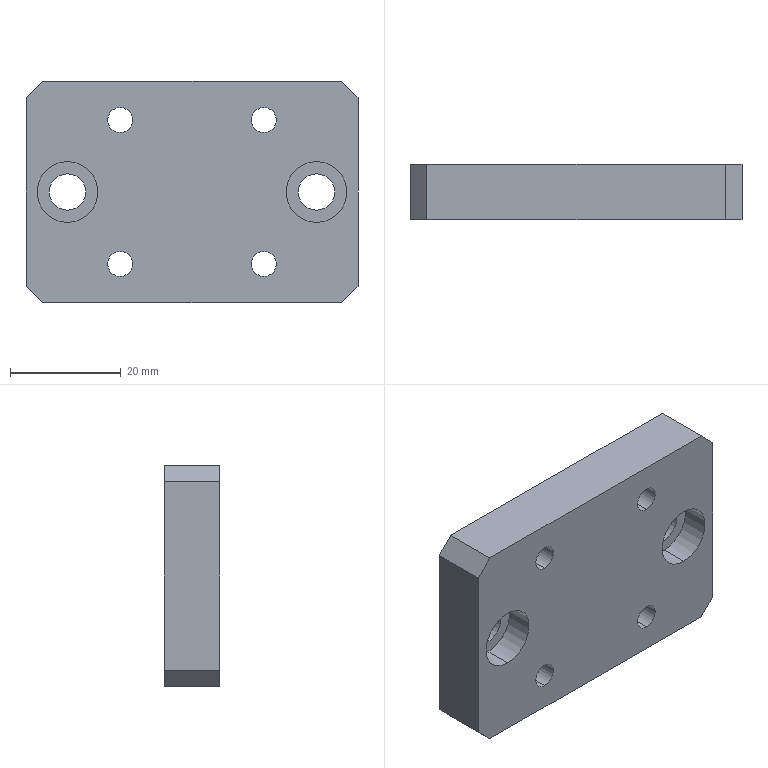Part | SolidWorks | features HoleWzd 2, Chamfer 1, Extrusion 1 | 1 solid | 40 faces | box 60 x 10 x 40 mm | volume 21259 mm3 | cylinder 24 | plane 16 | commonest cylinder face diameters 4.5 x8 8 x8 6.6 x4 11 x4
STEP:
#1=CARTESIAN_POINT('',(22.5,0.,5.5));
#2=VERTEX_POINT('',#1);
#3=CARTESIAN_POINT('',(22.5,0.,-5.5));
#4=VERTEX_POINT('',#3);
#5=CARTESIAN_POINT('',(22.5,0.,0.));
#6=DIRECTION('',(0.,-1.,0.));
#7=DIRECTION('',(0.,0.,-1.));
#8=AXIS2_PLACEMENT_3D('',#5,#6,#7);
#9=CIRCLE('',#8,5.5);
#10=EDGE_CURVE('',#2,#4,#9,.T.);
#11=ORIENTED_EDGE('',*,*,#10,.F.);
#12=CARTESIAN_POINT('',(22.5,-5.,5.5));
#13=VERTEX_POINT('',#12);
#14=CARTESIAN_POINT('',(22.5,-5.,5.5));
#15=DIRECTION('',(0.,-1.,0.));
#16=VECTOR('',#15,1000.);
#17=LINE('',#14,#16);
#18=EDGE_CURVE('',#2,#13,#17,.T.);
#19=ORIENTED_EDGE('',*,*,#18,.T.);
#20=CARTESIAN_POINT('',(22.5,-5.,-5.5));
#21=VERTEX_POINT('',#20);
#22=CARTESIAN_POINT('',(22.5,-5.,0.));
#23=DIRECTION('',(0.,-1.,0.));
#24=DIRECTION('',(0.,0.,-1.));
#25=AXIS2_PLACEMENT_3D('',#22,#23,#24);
#26=CIRCLE('',#25,5.5);
#27=EDGE_CURVE('',#13,#21,#26,.T.);
#28=ORIENTED_EDGE('',*,*,#27,.T.);
#29=CARTESIAN_POINT('',(22.5,-5.,-5.5));
#30=DIRECTION('',(0.,-1.,0.));
#31=VECTOR('',#30,1000.);
#32=LINE('',#29,#31);
#33=EDGE_CURVE('',#4,#21,#32,.T.);
#34=ORIENTED_EDGE('',*,*,#33,.F.);
#35=EDGE_LOOP('',(#11,#19,#28,#34));
#36=FACE_OUTER_BOUND('',#35,.T.);
#37=CARTESIAN_POINT('',(22.5,-5.,0.));
#38=DIRECTION('',(0.,-1.,0.));
#39=DIRECTION('',(0.,0.,-1.));
#40=AXIS2_PLACEMENT_3D('',#37,#38,#39);
#41=CYLINDRICAL_SURFACE('',#40,5.5);
#42=ADVANCED_FACE('',(#36),#41,.F.);
#43=CARTESIAN_POINT('',(22.5,5.,3.3));
#44=VERTEX_POINT('',#43);
#45=CARTESIAN_POINT('',(22.5,5.,-3.3));
#46=VERTEX_POINT('',#45);
#47=CARTESIAN_POINT('',(22.5,5.,0.));
#48=DIRECTION('',(0.,-1.,0.));
#49=DIRECTION('',(0.,0.,-1.));
#50=AXIS2_PLACEMENT_3D('',#47,#48,#49);
#51=CIRCLE('',#50,3.3);
#52=EDGE_CURVE('',#44,#46,#51,.T.);
#53=ORIENTED_EDGE('',*,*,#52,.F.);
#54=CARTESIAN_POINT('',(22.5,0.,3.3));
#55=VERTEX_POINT('',#54);
#56=CARTESIAN_POINT('',(22.5,-5.,3.3));
#57=DIRECTION('',(0.,-1.,0.));
#58=VECTOR('',#57,1000.);
#59=LINE('',#56,#58);
#60=EDGE_CURVE('',#44,#55,#59,.T.);
#61=ORIENTED_EDGE('',*,*,#60,.T.);
#62=CARTESIAN_POINT('',(22.5,0.,-3.3));
#63=VERTEX_POINT('',#62);
#64=CARTESIAN_POINT('',(22.5,0.,0.));
#65=DIRECTION('',(0.,-1.,0.));
#66=DIRECTION('',(0.,0.,-1.));
#67=AXIS2_PLACEMENT_3D('',#64,#65,#66);
#68=CIRCLE('',#67,3.3);
#69=EDGE_CURVE('',#55,#63,#68,.T.);
#70=ORIENTED_EDGE('',*,*,#69,.T.);
#71=CARTESIAN_POINT('',(22.5,-5.,-3.3));
#72=DIRECTION('',(0.,-1.,0.));
#73=VECTOR('',#72,1000.);
#74=LINE('',#71,#73);
#75=EDGE_CURVE('',#46,#63,#74,.T.);
#76=ORIENTED_EDGE('',*,*,#75,.F.);
#77=EDGE_LOOP('',(#53,#61,#70,#76));
#78=FACE_OUTER_BOUND('',#77,.T.);
#79=CARTESIAN_POINT('',(22.5,-5.,0.));
#80=DIRECTION('',(0.,-1.,0.));
#81=DIRECTION('',(0.,0.,-1.));
#82=AXIS2_PLACEMENT_3D('',#79,#80,#81);
#83=CYLINDRICAL_SURFACE('',#82,3.3);
#84=ADVANCED_FACE('',(#78),#83,.F.);
#85=CARTESIAN_POINT('',(-22.5,0.,5.5));
#86=VERTEX_POINT('',#85);
#87=CARTESIAN_POINT('',(-22.5,0.,-5.5));
#88=VERTEX_POINT('',#87);
#89=CARTESIAN_POINT('',(-22.5,0.,0.));
#90=DIRECTION('',(0.,-1.,0.));
#91=DIRECTION('',(0.,0.,-1.));
#92=AXIS2_PLACEMENT_3D('',#89,#90,#91);
#93=CIRCLE('',#92,5.5);
#94=EDGE_CURVE('',#86,#88,#93,.T.);
#95=ORIENTED_EDGE('',*,*,#94,.F.);
#96=CARTESIAN_POINT('',(-22.5,-5.,5.5));
#97=VERTEX_POINT('',#96);
#98=CARTESIAN_POINT('',(-22.5,-5.,5.5));
#99=DIRECTION('',(0.,-1.,0.));
#100=VECTOR('',#99,1000.);
#101=LINE('',#98,#100);
#102=EDGE_CURVE('',#86,#97,#101,.T.);
#103=ORIENTED_EDGE('',*,*,#102,.T.);
#104=CARTESIAN_POINT('',(-22.5,-5.,-5.5));
#105=VERTEX_POINT('',#104);
#106=CARTESIAN_POINT('',(-22.5,-5.,0.));
#107=DIRECTION('',(0.,-1.,0.));
#108=DIRECTION('',(0.,0.,-1.));
#109=AXIS2_PLACEMENT_3D('',#106,#107,#108);
#110=CIRCLE('',#109,5.5);
#111=EDGE_CURVE('',#97,#105,#110,.T.);
#112=ORIENTED_EDGE('',*,*,#111,.T.);
#113=CARTESIAN_POINT('',(-22.5,-5.,-5.5));
#114=DIRECTION('',(0.,-1.,0.));
#115=VECTOR('',#114,1000.);
#116=LINE('',#113,#115);
#117=EDGE_CURVE('',#88,#105,#116,.T.);
#118=ORIENTED_EDGE('',*,*,#117,.F.);
#119=EDGE_LOOP('',(#95,#103,#112,#118));
#120=FACE_OUTER_BOUND('',#119,.T.);
#121=CARTESIAN_POINT('',(-22.5,-5.,0.));
#122=DIRECTION('',(0.,-1.,0.));
#123=DIRECTION('',(0.,0.,-1.));
#124=AXIS2_PLACEMENT_3D('',#121,#122,#123);
#125=CYLINDRICAL_SURFACE('',#124,5.5);
#126=ADVANCED_FACE('',(#120),#125,.F.);
#127=CARTESIAN_POINT('',(-22.5,5.,3.3));
#128=VERTEX_POINT('',#127);
#129=CARTESIAN_POINT('',(-22.5,5.,-3.3));
#130=VERTEX_POINT('',#129);
#131=CARTESIAN_POINT('',(-22.5,5.,0.));
#132=DIRECTION('',(0.,-1.,0.));
#133=DIRECTION('',(0.,0.,-1.));
#134=AXIS2_PLACEMENT_3D('',#131,#132,#133);
#135=CIRCLE('',#134,3.3);
#136=EDGE_CURVE('',#128,#130,#135,.T.);
#137=ORIENTED_EDGE('',*,*,#136,.F.);
#138=CARTESIAN_POINT('',(-22.5,0.,3.3));
#139=VERTEX_POINT('',#138);
#140=CARTESIAN_POINT('',(-22.5,-5.,3.3));
#141=DIRECTION('',(0.,-1.,0.));
#142=VECTOR('',#141,1000.);
#143=LINE('',#140,#142);
#144=EDGE_CURVE('',#128,#139,#143,.T.);
#145=ORIENTED_EDGE('',*,*,#144,.T.);
#146=CARTESIAN_POINT('',(-22.5,0.,-3.3));
#147=VERTEX_POINT('',#146);
#148=CARTESIAN_POINT('',(-22.5,0.,0.));
#149=DIRECTION('',(0.,-1.,0.));
#150=DIRECTION('',(0.,0.,-1.));
#151=AXIS2_PLACEMENT_3D('',#148,#149,#150);
#152=CIRCLE('',#151,3.3);
#153=EDGE_CURVE('',#139,#147,#152,.T.);
#154=ORIENTED_EDGE('',*,*,#153,.T.);
#155=CARTESIAN_POINT('',(-22.5,-5.,-3.3));
#156=DIRECTION('',(0.,-1.,0.));
#157=VECTOR('',#156,1000.);
#158=LINE('',#155,#157);
#159=EDGE_CURVE('',#130,#147,#158,.T.);
#160=ORIENTED_EDGE('',*,*,#159,.F.);
#161=EDGE_LOOP('',(#137,#145,#154,#160));
#162=FACE_OUTER_BOUND('',#161,.T.);
#163=CARTESIAN_POINT('',(-22.5,-5.,0.));
#164=DIRECTION('',(0.,-1.,0.));
#165=DIRECTION('',(0.,0.,-1.));
#166=AXIS2_PLACEMENT_3D('',#163,#164,#165);
#167=CYLINDRICAL_SURFACE('',#166,3.3);
#168=ADVANCED_FACE('',(#162),#167,.F.);
#169=CARTESIAN_POINT('',(13.,0.4,9.));
#170=VERTEX_POINT('',#169);
#171=CARTESIAN_POINT('',(13.,0.4,17.));
#172=VERTEX_POINT('',#171);
#173=CARTESIAN_POINT('',(13.,0.4,13.));
#174=DIRECTION('',(0.,1.,0.));
#175=DIRECTION('',(0.,0.,1.));
#176=AXIS2_PLACEMENT_3D('',#173,#174,#175);
#177=CIRCLE('',#176,4.);
#178=EDGE_CURVE('',#170,#172,#177,.T.);
#179=ORIENTED_EDGE('',*,*,#178,.F.);
#180=CARTESIAN_POINT('',(13.,5.,9.));
#181=VERTEX_POINT('',#180);
#182=CARTESIAN_POINT('',(13.,5.,9.));
#183=DIRECTION('',(0.,1.,0.));
#184=VECTOR('',#183,1000.);
#185=LINE('',#182,#184);
#186=EDGE_CURVE('',#170,#181,#185,.T.);
#187=ORIENTED_EDGE('',*,*,#186,.T.);
#188=CARTESIAN_POINT('',(13.,5.,17.));
#189=VERTEX_POINT('',#188);
#190=CARTESIAN_POINT('',(13.,5.,13.));
#191=DIRECTION('',(0.,1.,0.));
#192=DIRECTION('',(0.,0.,1.));
#193=AXIS2_PLACEMENT_3D('',#190,#191,#192);
#194=CIRCLE('',#193,4.);
#195=EDGE_CURVE('',#181,#189,#194,.T.);
#196=ORIENTED_EDGE('',*,*,#195,.T.);
#197=CARTESIAN_POINT('',(13.,5.,17.));
#198=DIRECTION('',(0.,1.,0.));
#199=VECTOR('',#198,1000.);
#200=LINE('',#197,#199);
#201=EDGE_CURVE('',#172,#189,#200,.T.);
#202=ORIENTED_EDGE('',*,*,#201,.F.);
#203=EDGE_LOOP('',(#179,#187,#196,#202));
#204=FACE_OUTER_BOUND('',#203,.T.);
#205=CARTESIAN_POINT('',(13.,5.,13.));
#206=DIRECTION('',(0.,1.,0.));
#207=DIRECTION('',(0.,0.,1.));
#208=AXIS2_PLACEMENT_3D('',#205,#206,#207);
#209=CYLINDRICAL_SURFACE('',#208,4.);
#210=ADVANCED_FACE('',(#204),#209,.F.);
#211=CARTESIAN_POINT('',(13.,-5.,10.75));
#212=VERTEX_POINT('',#211);
#213=CARTESIAN_POINT('',(13.,-5.,15.25));
#214=VERTEX_POINT('',#213);
#215=CARTESIAN_POINT('',(13.,-5.,13.));
#216=DIRECTION('',(0.,1.,0.));
#217=DIRECTION('',(0.,0.,1.));
#218=AXIS2_PLACEMENT_3D('',#215,#216,#217);
#219=CIRCLE('',#218,2.25);
#220=EDGE_CURVE('',#212,#214,#219,.T.);
#221=ORIENTED_EDGE('',*,*,#220,.F.);
#222=CARTESIAN_POINT('',(13.,0.4,10.75));
#223=VERTEX_POINT('',#222);
#224=CARTESIAN_POINT('',(13.,5.,10.75));
#225=DIRECTION('',(0.,1.,0.));
#226=VECTOR('',#225,1000.);
#227=LINE('',#224,#226);
#228=EDGE_CURVE('',#212,#223,#227,.T.);
#229=ORIENTED_EDGE('',*,*,#228,.T.);
#230=CARTESIAN_POINT('',(13.,0.4,15.25));
#231=VERTEX_POINT('',#230);
#232=CARTESIAN_POINT('',(13.,0.4,13.));
#233=DIRECTION('',(0.,1.,0.));
#234=DIRECTION('',(0.,0.,1.));
#235=AXIS2_PLACEMENT_3D('',#232,#233,#234);
#236=CIRCLE('',#235,2.25);
#237=EDGE_CURVE('',#223,#231,#236,.T.);
#238=ORIENTED_EDGE('',*,*,#237,.T.);
#239=CARTESIAN_POINT('',(13.,5.,15.25));
#240=DIRECTION('',(0.,1.,0.));
#241=VECTOR('',#240,1000.);
#242=LINE('',#239,#241);
#243=EDGE_CURVE('',#214,#231,#242,.T.);
#244=ORIENTED_EDGE('',*,*,#243,.F.);
#245=EDGE_LOOP('',(#221,#229,#238,#244));
#246=FACE_OUTER_BOUND('',#245,.T.);
#247=CARTESIAN_POINT('',(13.,5.,13.));
#248=DIRECTION('',(0.,1.,0.));
#249=DIRECTION('',(0.,0.,1.));
#250=AXIS2_PLACEMENT_3D('',#247,#248,#249);
#251=CYLINDRICAL_SURFACE('',#250,2.25);
#252=ADVANCED_FACE('',(#246),#251,.F.);
#253=CARTESIAN_POINT('',(13.,0.4,-17.));
#254=VERTEX_POINT('',#253);
#255=CARTESIAN_POINT('',(13.,0.4,-9.));
#256=VERTEX_POINT('',#255);
#257=CARTESIAN_POINT('',(13.,0.4,-13.));
#258=DIRECTION('',(0.,1.,0.));
#259=DIRECTION('',(0.,0.,1.));
#260=AXIS2_PLACEMENT_3D('',#257,#258,#259);
#261=CIRCLE('',#260,4.);
#262=EDGE_CURVE('',#254,#256,#261,.T.);
#263=ORIENTED_EDGE('',*,*,#262,.F.);
#264=CARTESIAN_POINT('',(13.,5.,-17.));
#265=VERTEX_POINT('',#264);
#266=CARTESIAN_POINT('',(13.,5.,-17.));
#267=DIRECTION('',(0.,1.,0.));
#268=VECTOR('',#267,1000.);
#269=LINE('',#266,#268);
#270=EDGE_CURVE('',#254,#265,#269,.T.);
#271=ORIENTED_EDGE('',*,*,#270,.T.);
#272=CARTESIAN_POINT('',(13.,5.,-9.));
#273=VERTEX_POINT('',#272);
#274=CARTESIAN_POINT('',(13.,5.,-13.));
#275=DIRECTION('',(0.,1.,0.));
#276=DIRECTION('',(0.,0.,1.));
#277=AXIS2_PLACEMENT_3D('',#274,#275,#276);
#278=CIRCLE('',#277,4.);
#279=EDGE_CURVE('',#265,#273,#278,.T.);
#280=ORIENTED_EDGE('',*,*,#279,.T.);
#281=CARTESIAN_POINT('',(13.,5.,-9.));
#282=DIRECTION('',(0.,1.,0.));
#283=VECTOR('',#282,1000.);
#284=LINE('',#281,#283);
#285=EDGE_CURVE('',#256,#273,#284,.T.);
#286=ORIENTED_EDGE('',*,*,#285,.F.);
#287=EDGE_LOOP('',(#263,#271,#280,#286));
#288=FACE_OUTER_BOUND('',#287,.T.);
#289=CARTESIAN_POINT('',(13.,5.,-13.));
#290=DIRECTION('',(0.,1.,0.));
#291=DIRECTION('',(0.,0.,1.));
#292=AXIS2_PLACEMENT_3D('',#289,#290,#291);
#293=CYLINDRICAL_SURFACE('',#292,4.);
#294=ADVANCED_FACE('',(#288),#293,.F.);
#295=CARTESIAN_POINT('',(13.,-5.,-15.25));
#296=VERTEX_POINT('',#295);
#297=CARTESIAN_POINT('',(13.,-5.,-10.75));
#298=VERTEX_POINT('',#297);
#299=CARTESIAN_POINT('',(13.,-5.,-13.));
#300=DIRECTION('',(0.,1.,0.));
#301=DIRECTION('',(0.,0.,1.));
#302=AXIS2_PLACEMENT_3D('',#299,#300,#301);
#303=CIRCLE('',#302,2.25);
#304=EDGE_CURVE('',#296,#298,#303,.T.);
#305=ORIENTED_EDGE('',*,*,#304,.F.);
#306=CARTESIAN_POINT('',(13.,0.4,-15.25));
#307=VERTEX_POINT('',#306);
#308=CARTESIAN_POINT('',(13.,5.,-15.25));
#309=DIRECTION('',(0.,1.,0.));
#310=VECTOR('',#309,1000.);
#311=LINE('',#308,#310);
#312=EDGE_CURVE('',#296,#307,#311,.T.);
#313=ORIENTED_EDGE('',*,*,#312,.T.);
#314=CARTESIAN_POINT('',(13.,0.4,-10.75));
#315=VERTEX_POINT('',#314);
#316=CARTESIAN_POINT('',(13.,0.4,-13.));
#317=DIRECTION('',(0.,1.,0.));
#318=DIRECTION('',(0.,0.,1.));
#319=AXIS2_PLACEMENT_3D('',#316,#317,#318);
#320=CIRCLE('',#319,2.25);
#321=EDGE_CURVE('',#307,#315,#320,.T.);
#322=ORIENTED_EDGE('',*,*,#321,.T.);
#323=CARTESIAN_POINT('',(13.,5.,-10.75));
#324=DIRECTION('',(0.,1.,0.));
#325=VECTOR('',#324,1000.);
#326=LINE('',#323,#325);
#327=EDGE_CURVE('',#298,#315,#326,.T.);
#328=ORIENTED_EDGE('',*,*,#327,.F.);
#329=EDGE_LOOP('',(#305,#313,#322,#328));
#330=FACE_OUTER_BOUND('',#329,.T.);
#331=CARTESIAN_POINT('',(13.,5.,-13.));
#332=DIRECTION('',(0.,1.,0.));
#333=DIRECTION('',(0.,0.,1.));
#334=AXIS2_PLACEMENT_3D('',#331,#332,#333);
#335=CYLINDRICAL_SURFACE('',#334,2.25);
#336=ADVANCED_FACE('',(#330),#335,.F.);
#337=CARTESIAN_POINT('',(-13.,0.4,-17.));
#338=VERTEX_POINT('',#337);
#339=CARTESIAN_POINT('',(-13.,0.4,-9.));
#340=VERTEX_POINT('',#339);
#341=CARTESIAN_POINT('',(-13.,0.4,-13.));
#342=DIRECTION('',(0.,1.,0.));
#343=DIRECTION('',(0.,0.,1.));
#344=AXIS2_PLACEMENT_3D('',#341,#342,#343);
#345=CIRCLE('',#344,4.);
#346=EDGE_CURVE('',#338,#340,#345,.T.);
#347=ORIENTED_EDGE('',*,*,#346,.F.);
#348=CARTESIAN_POINT('',(-13.,5.,-17.));
#349=VERTEX_POINT('',#348);
#350=CARTESIAN_POINT('',(-13.,5.,-17.));
#351=DIRECTION('',(0.,1.,0.));
#352=VECTOR('',#351,1000.);
#353=LINE('',#350,#352);
#354=EDGE_CURVE('',#338,#349,#353,.T.);
#355=ORIENTED_EDGE('',*,*,#354,.T.);
#356=CARTESIAN_POINT('',(-13.,5.,-9.));
#357=VERTEX_POINT('',#356);
#358=CARTESIAN_POINT('',(-13.,5.,-13.));
#359=DIRECTION('',(0.,1.,0.));
#360=DIRECTION('',(0.,0.,1.));
#361=AXIS2_PLACEMENT_3D('',#358,#359,#360);
#362=CIRCLE('',#361,4.);
#363=EDGE_CURVE('',#349,#357,#362,.T.);
#364=ORIENTED_EDGE('',*,*,#363,.T.);
#365=CARTESIAN_POINT('',(-13.,5.,-9.));
#366=DIRECTION('',(0.,1.,0.));
#367=VECTOR('',#366,1000.);
#368=LINE('',#365,#367);
#369=EDGE_CURVE('',#340,#357,#368,.T.);
#370=ORIENTED_EDGE('',*,*,#369,.F.);
#371=EDGE_LOOP('',(#347,#355,#364,#370));
#372=FACE_OUTER_BOUND('',#371,.T.);
#373=CARTESIAN_POINT('',(-13.,5.,-13.));
#374=DIRECTION('',(0.,1.,0.));
#375=DIRECTION('',(0.,0.,1.));
#376=AXIS2_PLACEMENT_3D('',#373,#374,#375);
#377=CYLINDRICAL_SURFACE('',#376,4.);
#378=ADVANCED_FACE('',(#372),#377,.F.);
#379=CARTESIAN_POINT('',(-13.,-5.,-15.25));
#380=VERTEX_POINT('',#379);
#381=CARTESIAN_POINT('',(-13.,-5.,-10.75));
#382=VERTEX_POINT('',#381);
#383=CARTESIAN_POINT('',(-13.,-5.,-13.));
#384=DIRECTION('',(0.,1.,0.));
#385=DIRECTION('',(0.,0.,1.));
#386=AXIS2_PLACEMENT_3D('',#383,#384,#385);
#387=CIRCLE('',#386,2.25);
#388=EDGE_CURVE('',#380,#382,#387,.T.);
#389=ORIENTED_EDGE('',*,*,#388,.F.);
#390=CARTESIAN_POINT('',(-13.,0.4,-15.25));
#391=VERTEX_POINT('',#390);
#392=CARTESIAN_POINT('',(-13.,5.,-15.25));
#393=DIRECTION('',(0.,1.,0.));
#394=VECTOR('',#393,1000.);
#395=LINE('',#392,#394);
#396=EDGE_CURVE('',#380,#391,#395,.T.);
#397=ORIENTED_EDGE('',*,*,#396,.T.);
#398=CARTESIAN_POINT('',(-13.,0.4,-10.75));
#399=VERTEX_POINT('',#398);
#400=CARTESIAN_POINT('',(-13.,0.4,-13.));
#401=DIRECTION('',(0.,1.,0.));
#402=DIRECTION('',(0.,0.,1.));
#403=AXIS2_PLACEMENT_3D('',#400,#401,#402);
#404=CIRCLE('',#403,2.25);
#405=EDGE_CURVE('',#391,#399,#404,.T.);
#406=ORIENTED_EDGE('',*,*,#405,.T.);
#407=CARTESIAN_POINT('',(-13.,5.,-10.75));
#408=DIRECTION('',(0.,1.,0.));
#409=VECTOR('',#408,1000.);
#410=LINE('',#407,#409);
#411=EDGE_CURVE('',#382,#399,#410,.T.);
#412=ORIENTED_EDGE('',*,*,#411,.F.);
#413=EDGE_LOOP('',(#389,#397,#406,#412));
#414=FACE_OUTER_BOUND('',#413,.T.);
#415=CARTESIAN_POINT('',(-13.,5.,-13.));
#416=DIRECTION('',(0.,1.,0.));
#417=DIRECTION('',(0.,0.,1.));
#418=AXIS2_PLACEMENT_3D('',#415,#416,#417);
#419=CYLINDRICAL_SURFACE('',#418,2.25);
#420=ADVANCED_FACE('',(#414),#419,.F.);
#421=CARTESIAN_POINT('',(-13.,0.4,9.));
#422=VERTEX_POINT('',#421);
#423=CARTESIAN_POINT('',(-13.,0.4,17.));
#424=VERTEX_POINT('',#423);
#425=CARTESIAN_POINT('',(-13.,0.4,13.));
#426=DIRECTION('',(0.,1.,0.));
#427=DIRECTION('',(0.,0.,1.));
#428=AXIS2_PLACEMENT_3D('',#425,#426,#427);
#429=CIRCLE('',#428,4.);
#430=EDGE_CURVE('',#422,#424,#429,.T.);
#431=ORIENTED_EDGE('',*,*,#430,.F.);
#432=CARTESIAN_POINT('',(-13.,5.,9.));
#433=VERTEX_POINT('',#432);
#434=CARTESIAN_POINT('',(-13.,5.,9.));
#435=DIRECTION('',(0.,1.,0.));
#436=VECTOR('',#435,1000.);
#437=LINE('',#434,#436);
#438=EDGE_CURVE('',#422,#433,#437,.T.);
#439=ORIENTED_EDGE('',*,*,#438,.T.);
#440=CARTESIAN_POINT('',(-13.,5.,17.));
#441=VERTEX_POINT('',#440);
#442=CARTESIAN_POINT('',(-13.,5.,13.));
#443=DIRECTION('',(0.,1.,0.));
#444=DIRECTION('',(0.,0.,1.));
#445=AXIS2_PLACEMENT_3D('',#442,#443,#444);
#446=CIRCLE('',#445,4.);
#447=EDGE_CURVE('',#433,#441,#446,.T.);
#448=ORIENTED_EDGE('',*,*,#447,.T.);
#449=CARTESIAN_POINT('',(-13.,5.,17.));
#450=DIRECTION('',(0.,1.,0.));
#451=VECTOR('',#450,1000.);
#452=LINE('',#449,#451);
#453=EDGE_CURVE('',#424,#441,#452,.T.);
#454=ORIENTED_EDGE('',*,*,#453,.F.);
#455=EDGE_LOOP('',(#431,#439,#448,#454));
#456=FACE_OUTER_BOUND('',#455,.T.);
#457=CARTESIAN_POINT('',(-13.,5.,13.));
#458=DIRECTION('',(0.,1.,0.));
#459=DIRECTION('',(0.,0.,1.));
#460=AXIS2_PLACEMENT_3D('',#457,#458,#459);
#461=CYLINDRICAL_SURFACE('',#460,4.);
#462=ADVANCED_FACE('',(#456),#461,.F.);
#463=CARTESIAN_POINT('',(-13.,-5.,10.75));
#464=VERTEX_POINT('',#463);
#465=CARTESIAN_POINT('',(-13.,-5.,15.25));
#466=VERTEX_POINT('',#465);
#467=CARTESIAN_POINT('',(-13.,-5.,13.));
#468=DIRECTION('',(0.,1.,0.));
#469=DIRECTION('',(0.,0.,1.));
#470=AXIS2_PLACEMENT_3D('',#467,#468,#469);
#471=CIRCLE('',#470,2.25);
#472=EDGE_CURVE('',#464,#466,#471,.T.);
#473=ORIENTED_EDGE('',*,*,#472,.F.);
#474=CARTESIAN_POINT('',(-13.,0.4,10.75));
#475=VERTEX_POINT('',#474);
#476=CARTESIAN_POINT('',(-13.,5.,10.75));
#477=DIRECTION('',(0.,1.,0.));
#478=VECTOR('',#477,1000.);
#479=LINE('',#476,#478);
#480=EDGE_CURVE('',#464,#475,#479,.T.);
#481=ORIENTED_EDGE('',*,*,#480,.T.);
#482=CARTESIAN_POINT('',(-13.,0.4,15.25));
#483=VERTEX_POINT('',#482);
#484=CARTESIAN_POINT('',(-13.,0.4,13.));
#485=DIRECTION('',(0.,1.,0.));
#486=DIRECTION('',(0.,0.,1.));
#487=AXIS2_PLACEMENT_3D('',#484,#485,#486);
#488=CIRCLE('',#487,2.25);
#489=EDGE_CURVE('',#475,#483,#488,.T.);
#490=ORIENTED_EDGE('',*,*,#489,.T.);
#491=CARTESIAN_POINT('',(-13.,5.,15.25));
#492=DIRECTION('',(0.,1.,0.));
#493=VECTOR('',#492,1000.);
#494=LINE('',#491,#493);
#495=EDGE_CURVE('',#466,#483,#494,.T.);
#496=ORIENTED_EDGE('',*,*,#495,.F.);
#497=EDGE_LOOP('',(#473,#481,#490,#496));
#498=FACE_OUTER_BOUND('',#497,.T.);
#499=CARTESIAN_POINT('',(-13.,5.,13.));
#500=DIRECTION('',(0.,1.,0.));
#501=DIRECTION('',(0.,0.,1.));
#502=AXIS2_PLACEMENT_3D('',#499,#500,#501);
#503=CYLINDRICAL_SURFACE('',#502,2.25);
#504=ADVANCED_FACE('',(#498),#503,.F.);
#505=CARTESIAN_POINT('',(30.,5.,17.));
#506=VERTEX_POINT('',#505);
#507=CARTESIAN_POINT('',(30.,5.,-17.));
#508=VERTEX_POINT('',#507);
#509=CARTESIAN_POINT('',(30.,5.,20.));
#510=DIRECTION('',(0.,0.,-1.));
#511=VECTOR('',#510,1000.);
#512=LINE('',#509,#511);
#513=EDGE_CURVE('',#506,#508,#512,.T.);
#514=ORIENTED_EDGE('',*,*,#513,.F.);
#515=CARTESIAN_POINT('',(30.,-5.,17.));
#516=VERTEX_POINT('',#515);
#517=CARTESIAN_POINT('',(30.,5.,17.));
#518=DIRECTION('',(0.,-1.,0.));
#519=VECTOR('',#518,1000.);
#520=LINE('',#517,#519);
#521=EDGE_CURVE('',#506,#516,#520,.T.);
#522=ORIENTED_EDGE('',*,*,#521,.T.);
#523=CARTESIAN_POINT('',(30.,-5.,-17.));
#524=VERTEX_POINT('',#523);
#525=CARTESIAN_POINT('',(30.,-5.,20.));
#526=DIRECTION('',(0.,0.,-1.));
#527=VECTOR('',#526,1000.);
#528=LINE('',#525,#527);
#529=EDGE_CURVE('',#516,#524,#528,.T.);
#530=ORIENTED_EDGE('',*,*,#529,.T.);
#531=CARTESIAN_POINT('',(30.,5.,-17.));
#532=DIRECTION('',(0.,1.,0.));
#533=VECTOR('',#532,1000.);
#534=LINE('',#531,#533);
#535=EDGE_CURVE('',#524,#508,#534,.T.);
#536=ORIENTED_EDGE('',*,*,#535,.T.);
#537=EDGE_LOOP('',(#514,#522,#530,#536));
#538=FACE_OUTER_BOUND('',#537,.T.);
#539=CARTESIAN_POINT('',(30.,5.,20.));
#540=DIRECTION('',(-1.,0.,0.));
#541=DIRECTION('',(0.,0.,1.));
#542=AXIS2_PLACEMENT_3D('',#539,#540,#541);
#543=PLANE('',#542);
#544=ADVANCED_FACE('',(#538),#543,.F.);
#545=CARTESIAN_POINT('',(27.,5.,-20.));
#546=VERTEX_POINT('',#545);
#547=CARTESIAN_POINT('',(-27.,5.,-20.));
#548=VERTEX_POINT('',#547);
#549=CARTESIAN_POINT('',(-30.,5.,-20.));
#550=DIRECTION('',(-1.,0.,0.));
#551=VECTOR('',#550,1000.);
#552=LINE('',#549,#551);
#553=EDGE_CURVE('',#546,#548,#552,.T.);
#554=ORIENTED_EDGE('',*,*,#553,.F.);
#555=CARTESIAN_POINT('',(27.,-5.,-20.));
#556=VERTEX_POINT('',#555);
#557=CARTESIAN_POINT('',(27.,5.,-20.));
#558=DIRECTION('',(0.,-1.,0.));
#559=VECTOR('',#558,1000.);
#560=LINE('',#557,#559);
#561=EDGE_CURVE('',#546,#556,#560,.T.);
#562=ORIENTED_EDGE('',*,*,#561,.T.);
#563=CARTESIAN_POINT('',(-27.,-5.,-20.));
#564=VERTEX_POINT('',#563);
#565=CARTESIAN_POINT('',(-30.,-5.,-20.));
#566=DIRECTION('',(-1.,0.,0.));
#567=VECTOR('',#566,1000.);
#568=LINE('',#565,#567);
#569=EDGE_CURVE('',#556,#564,#568,.T.);
#570=ORIENTED_EDGE('',*,*,#569,.T.);
#571=CARTESIAN_POINT('',(-27.,5.,-20.));
#572=DIRECTION('',(0.,1.,0.));
#573=VECTOR('',#572,1000.);
#574=LINE('',#571,#573);
#575=EDGE_CURVE('',#564,#548,#574,.T.);
#576=ORIENTED_EDGE('',*,*,#575,.T.);
#577=EDGE_LOOP('',(#554,#562,#570,#576));
#578=FACE_OUTER_BOUND('',#577,.T.);
#579=CARTESIAN_POINT('',(-30.,5.,-20.));
#580=DIRECTION('',(0.,0.,1.));
#581=DIRECTION('',(1.,0.,0.));
#582=AXIS2_PLACEMENT_3D('',#579,#580,#581);
#583=PLANE('',#582);
#584=ADVANCED_FACE('',(#578),#583,.F.);
#585=CARTESIAN_POINT('',(-30.,5.,-17.));
#586=VERTEX_POINT('',#585);
#587=CARTESIAN_POINT('',(-30.,5.,17.));
#588=VERTEX_POINT('',#587);
#589=CARTESIAN_POINT('',(-30.,5.,20.));
#590=DIRECTION('',(0.,0.,1.));
#591=VECTOR('',#590,1000.);
#592=LINE('',#589,#591);
#593=EDGE_CURVE('',#586,#588,#592,.T.);
#594=ORIENTED_EDGE('',*,*,#593,.F.);
#595=CARTESIAN_POINT('',(-30.,-5.,-17.));
#596=VERTEX_POINT('',#595);
#597=CARTESIAN_POINT('',(-30.,5.,-17.));
#598=DIRECTION('',(0.,-1.,0.));
#599=VECTOR('',#598,1000.);
#600=LINE('',#597,#599);
#601=EDGE_CURVE('',#586,#596,#600,.T.);
#602=ORIENTED_EDGE('',*,*,#601,.T.);
#603=CARTESIAN_POINT('',(-30.,-5.,17.));
#604=VERTEX_POINT('',#603);
#605=CARTESIAN_POINT('',(-30.,-5.,20.));
#606=DIRECTION('',(0.,0.,1.));
#607=VECTOR('',#606,1000.);
#608=LINE('',#605,#607);
#609=EDGE_CURVE('',#596,#604,#608,.T.);
#610=ORIENTED_EDGE('',*,*,#609,.T.);
#611=CARTESIAN_POINT('',(-30.,5.,17.));
#612=DIRECTION('',(0.,1.,0.));
#613=VECTOR('',#612,1000.);
#614=LINE('',#611,#613);
#615=EDGE_CURVE('',#604,#588,#614,.T.);
#616=ORIENTED_EDGE('',*,*,#615,.T.);
#617=EDGE_LOOP('',(#594,#602,#610,#616));
#618=FACE_OUTER_BOUND('',#617,.T.);
#619=CARTESIAN_POINT('',(-30.,5.,20.));
#620=DIRECTION('',(1.,0.,0.));
#621=DIRECTION('',(0.,0.,-1.));
#622=AXIS2_PLACEMENT_3D('',#619,#620,#621);
#623=PLANE('',#622);
#624=ADVANCED_FACE('',(#618),#623,.F.);
#625=CARTESIAN_POINT('',(-27.,-5.,20.));
#626=VERTEX_POINT('',#625);
#627=CARTESIAN_POINT('',(27.,-5.,20.));
#628=VERTEX_POINT('',#627);
#629=CARTESIAN_POINT('',(-30.,-5.,20.));
#630=DIRECTION('',(1.,0.,0.));
#631=VECTOR('',#630,1000.);
#632=LINE('',#629,#631);
#633=EDGE_CURVE('',#626,#628,#632,.T.);
#634=ORIENTED_EDGE('',*,*,#633,.T.);
#635=CARTESIAN_POINT('',(27.,5.,20.));
#636=VERTEX_POINT('',#635);
#637=CARTESIAN_POINT('',(27.,5.,20.));
#638=DIRECTION('',(0.,1.,0.));
#639=VECTOR('',#638,1000.);
#640=LINE('',#637,#639);
#641=EDGE_CURVE('',#628,#636,#640,.T.);
#642=ORIENTED_EDGE('',*,*,#641,.T.);
#643=CARTESIAN_POINT('',(-27.,5.,20.));
#644=VERTEX_POINT('',#643);
#645=CARTESIAN_POINT('',(-30.,5.,20.));
#646=DIRECTION('',(1.,0.,0.));
#647=VECTOR('',#646,1000.);
#648=LINE('',#645,#647);
#649=EDGE_CURVE('',#644,#636,#648,.T.);
#650=ORIENTED_EDGE('',*,*,#649,.F.);
#651=CARTESIAN_POINT('',(-27.,5.,20.));
#652=DIRECTION('',(0.,-1.,0.));
#653=VECTOR('',#652,1000.);
#654=LINE('',#651,#653);
#655=EDGE_CURVE('',#644,#626,#654,.T.);
#656=ORIENTED_EDGE('',*,*,#655,.T.);
#657=EDGE_LOOP('',(#634,#642,#650,#656));
#658=FACE_OUTER_BOUND('',#657,.T.);
#659=CARTESIAN_POINT('',(-30.,5.,20.));
#660=DIRECTION('',(0.,0.,-1.));
#661=DIRECTION('',(-1.,0.,0.));
#662=AXIS2_PLACEMENT_3D('',#659,#660,#661);
#663=PLANE('',#662);
#664=ADVANCED_FACE('',(#658),#663,.F.);
#665=CARTESIAN_POINT('',(22.5,5.,0.));
#666=DIRECTION('',(0.,-1.,0.));
#667=DIRECTION('',(0.,0.,-1.));
#668=AXIS2_PLACEMENT_3D('',#665,#666,#667);
#669=CIRCLE('',#668,3.3);
#670=EDGE_CURVE('',#46,#44,#669,.T.);
#671=ORIENTED_EDGE('',*,*,#670,.T.);
#672=ORIENTED_EDGE('',*,*,#52,.T.);
#673=EDGE_LOOP('',(#671,#672));
#674=FACE_BOUND('',#673,.T.);
#675=CARTESIAN_POINT('',(-22.5,5.,0.));
#676=DIRECTION('',(0.,-1.,0.));
#677=DIRECTION('',(0.,0.,-1.));
#678=AXIS2_PLACEMENT_3D('',#675,#676,#677);
#679=CIRCLE('',#678,3.3);
#680=EDGE_CURVE('',#130,#128,#679,.T.);
#681=ORIENTED_EDGE('',*,*,#680,.T.);
#682=ORIENTED_EDGE('',*,*,#136,.T.);
#683=EDGE_LOOP('',(#681,#682));
#684=FACE_BOUND('',#683,.T.);
#685=CARTESIAN_POINT('',(13.,5.,13.));
#686=DIRECTION('',(0.,1.,0.));
#687=DIRECTION('',(0.,0.,1.));
#688=AXIS2_PLACEMENT_3D('',#685,#686,#687);
#689=CIRCLE('',#688,4.);
#690=EDGE_CURVE('',#189,#181,#689,.T.);
#691=ORIENTED_EDGE('',*,*,#690,.F.);
#692=ORIENTED_EDGE('',*,*,#195,.F.);
#693=EDGE_LOOP('',(#691,#692));
#694=FACE_BOUND('',#693,.T.);
#695=CARTESIAN_POINT('',(13.,5.,-13.));
#696=DIRECTION('',(0.,1.,0.));
#697=DIRECTION('',(0.,0.,1.));
#698=AXIS2_PLACEMENT_3D('',#695,#696,#697);
#699=CIRCLE('',#698,4.);
#700=EDGE_CURVE('',#273,#265,#699,.T.);
#701=ORIENTED_EDGE('',*,*,#700,.F.);
#702=ORIENTED_EDGE('',*,*,#279,.F.);
#703=EDGE_LOOP('',(#701,#702));
#704=FACE_BOUND('',#703,.T.);
#705=CARTESIAN_POINT('',(-13.,5.,-13.));
#706=DIRECTION('',(0.,1.,0.));
#707=DIRECTION('',(0.,0.,1.));
#708=AXIS2_PLACEMENT_3D('',#705,#706,#707);
#709=CIRCLE('',#708,4.);
#710=EDGE_CURVE('',#357,#349,#709,.T.);
#711=ORIENTED_EDGE('',*,*,#710,.F.);
#712=ORIENTED_EDGE('',*,*,#363,.F.);
#713=EDGE_LOOP('',(#711,#712));
#714=FACE_BOUND('',#713,.T.);
#715=CARTESIAN_POINT('',(-13.,5.,13.));
#716=DIRECTION('',(0.,1.,0.));
#717=DIRECTION('',(0.,0.,1.));
#718=AXIS2_PLACEMENT_3D('',#715,#716,#717);
#719=CIRCLE('',#718,4.);
#720=EDGE_CURVE('',#441,#433,#719,.T.);
#721=ORIENTED_EDGE('',*,*,#720,.F.);
#722=ORIENTED_EDGE('',*,*,#447,.F.);
#723=EDGE_LOOP('',(#721,#722));
#724=FACE_BOUND('',#723,.T.);
#725=ORIENTED_EDGE('',*,*,#649,.T.);
#726=CARTESIAN_POINT('',(30.,5.,17.));
#727=DIRECTION('',(0.7071,0.,-0.7071));
#728=VECTOR('',#727,1000.);
#729=LINE('',#726,#728);
#730=EDGE_CURVE('',#636,#506,#729,.T.);
#731=ORIENTED_EDGE('',*,*,#730,.T.);
#732=ORIENTED_EDGE('',*,*,#513,.T.);
#733=CARTESIAN_POINT('',(27.,5.,-20.));
#734=DIRECTION('',(-0.7071,0.,-0.7071));
#735=VECTOR('',#734,1000.);
#736=LINE('',#733,#735);
#737=EDGE_CURVE('',#508,#546,#736,.T.);
#738=ORIENTED_EDGE('',*,*,#737,.T.);
#739=ORIENTED_EDGE('',*,*,#553,.T.);
#740=CARTESIAN_POINT('',(-30.,5.,-17.));
#741=DIRECTION('',(-0.7071,0.,0.7071));
#742=VECTOR('',#741,1000.);
#743=LINE('',#740,#742);
#744=EDGE_CURVE('',#548,#586,#743,.T.);
#745=ORIENTED_EDGE('',*,*,#744,.T.);
#746=ORIENTED_EDGE('',*,*,#593,.T.);
#747=CARTESIAN_POINT('',(-27.,5.,20.));
#748=DIRECTION('',(0.7071,0.,0.7071));
#749=VECTOR('',#748,1000.);
#750=LINE('',#747,#749);
#751=EDGE_CURVE('',#588,#644,#750,.T.);
#752=ORIENTED_EDGE('',*,*,#751,.T.);
#753=EDGE_LOOP('',(#725,#731,#732,#738,#739,#745,#746,#752));
#754=FACE_OUTER_BOUND('',#753,.T.);
#755=CARTESIAN_POINT('',(0.,5.,0.));
#756=DIRECTION('',(0.,-1.,0.));
#757=DIRECTION('',(0.,0.,-1.));
#758=AXIS2_PLACEMENT_3D('',#755,#756,#757);
#759=PLANE('',#758);
#760=ADVANCED_FACE('',(#674,#684,#694,#704,#714,#724,#754),#759,.F.);
#761=CARTESIAN_POINT('',(22.5,-5.,0.));
#762=DIRECTION('',(0.,-1.,0.));
#763=DIRECTION('',(0.,0.,-1.));
#764=AXIS2_PLACEMENT_3D('',#761,#762,#763);
#765=CIRCLE('',#764,5.5);
#766=EDGE_CURVE('',#21,#13,#765,.T.);
#767=ORIENTED_EDGE('',*,*,#766,.F.);
#768=ORIENTED_EDGE('',*,*,#27,.F.);
#769=EDGE_LOOP('',(#767,#768));
#770=FACE_BOUND('',#769,.T.);
#771=CARTESIAN_POINT('',(-22.5,-5.,0.));
#772=DIRECTION('',(0.,-1.,0.));
#773=DIRECTION('',(0.,0.,-1.));
#774=AXIS2_PLACEMENT_3D('',#771,#772,#773);
#775=CIRCLE('',#774,5.5);
#776=EDGE_CURVE('',#105,#97,#775,.T.);
#777=ORIENTED_EDGE('',*,*,#776,.F.);
#778=ORIENTED_EDGE('',*,*,#111,.F.);
#779=EDGE_LOOP('',(#777,#778));
#780=FACE_BOUND('',#779,.T.);
#781=CARTESIAN_POINT('',(13.,-5.,13.));
#782=DIRECTION('',(0.,1.,0.));
#783=DIRECTION('',(0.,0.,1.));
#784=AXIS2_PLACEMENT_3D('',#781,#782,#783);
#785=CIRCLE('',#784,2.25);
#786=EDGE_CURVE('',#214,#212,#785,.T.);
#787=ORIENTED_EDGE('',*,*,#786,.T.);
#788=ORIENTED_EDGE('',*,*,#220,.T.);
#789=EDGE_LOOP('',(#787,#788));
#790=FACE_BOUND('',#789,.T.);
#791=CARTESIAN_POINT('',(13.,-5.,-13.));
#792=DIRECTION('',(0.,1.,0.));
#793=DIRECTION('',(0.,0.,1.));
#794=AXIS2_PLACEMENT_3D('',#791,#792,#793);
#795=CIRCLE('',#794,2.25);
#796=EDGE_CURVE('',#298,#296,#795,.T.);
#797=ORIENTED_EDGE('',*,*,#796,.T.);
#798=ORIENTED_EDGE('',*,*,#304,.T.);
#799=EDGE_LOOP('',(#797,#798));
#800=FACE_BOUND('',#799,.T.);
#801=CARTESIAN_POINT('',(-13.,-5.,-13.));
#802=DIRECTION('',(0.,1.,0.));
#803=DIRECTION('',(0.,0.,1.));
#804=AXIS2_PLACEMENT_3D('',#801,#802,#803);
#805=CIRCLE('',#804,2.25);
#806=EDGE_CURVE('',#382,#380,#805,.T.);
#807=ORIENTED_EDGE('',*,*,#806,.T.);
#808=ORIENTED_EDGE('',*,*,#388,.T.);
#809=EDGE_LOOP('',(#807,#808));
#810=FACE_BOUND('',#809,.T.);
#811=CARTESIAN_POINT('',(-13.,-5.,13.));
#812=DIRECTION('',(0.,1.,0.));
#813=DIRECTION('',(0.,0.,1.));
#814=AXIS2_PLACEMENT_3D('',#811,#812,#813);
#815=CIRCLE('',#814,2.25);
#816=EDGE_CURVE('',#466,#464,#815,.T.);
#817=ORIENTED_EDGE('',*,*,#816,.T.);
#818=ORIENTED_EDGE('',*,*,#472,.T.);
#819=EDGE_LOOP('',(#817,#818));
#820=FACE_BOUND('',#819,.T.);
#821=ORIENTED_EDGE('',*,*,#529,.F.);
#822=CARTESIAN_POINT('',(23.5,-5.,23.5));
#823=DIRECTION('',(-0.7071,0.,0.7071));
#824=VECTOR('',#823,1000.);
#825=LINE('',#822,#824);
#826=EDGE_CURVE('',#516,#628,#825,.T.);
#827=ORIENTED_EDGE('',*,*,#826,.T.);
#828=ORIENTED_EDGE('',*,*,#633,.F.);
#829=CARTESIAN_POINT('',(-23.5,-5.,23.5));
#830=DIRECTION('',(-0.7071,0.,-0.7071));
#831=VECTOR('',#830,1000.);
#832=LINE('',#829,#831);
#833=EDGE_CURVE('',#626,#604,#832,.T.);
#834=ORIENTED_EDGE('',*,*,#833,.T.);
#835=ORIENTED_EDGE('',*,*,#609,.F.);
#836=CARTESIAN_POINT('',(-23.5,-5.,-23.5));
#837=DIRECTION('',(0.7071,0.,-0.7071));
#838=VECTOR('',#837,1000.);
#839=LINE('',#836,#838);
#840=EDGE_CURVE('',#596,#564,#839,.T.);
#841=ORIENTED_EDGE('',*,*,#840,.T.);
#842=ORIENTED_EDGE('',*,*,#569,.F.);
#843=CARTESIAN_POINT('',(23.5,-5.,-23.5));
#844=DIRECTION('',(0.7071,0.,0.7071));
#845=VECTOR('',#844,1000.);
#846=LINE('',#843,#845);
#847=EDGE_CURVE('',#556,#524,#846,.T.);
#848=ORIENTED_EDGE('',*,*,#847,.T.);
#849=EDGE_LOOP('',(#821,#827,#828,#834,#835,#841,#842,#848));
#850=FACE_OUTER_BOUND('',#849,.T.);
#851=CARTESIAN_POINT('',(0.,-5.,0.));
#852=DIRECTION('',(0.,-1.,0.));
#853=DIRECTION('',(0.,0.,-1.));
#854=AXIS2_PLACEMENT_3D('',#851,#852,#853);
#855=PLANE('',#854);
#856=ADVANCED_FACE('',(#770,#780,#790,#800,#810,#820,#850),#855,.T.);
#857=ORIENTED_EDGE('',*,*,#480,.F.);
#858=ORIENTED_EDGE('',*,*,#816,.F.);
#859=ORIENTED_EDGE('',*,*,#495,.T.);
#860=CARTESIAN_POINT('',(-13.,0.4,13.));
#861=DIRECTION('',(0.,1.,0.));
#862=DIRECTION('',(0.,0.,1.));
#863=AXIS2_PLACEMENT_3D('',#860,#861,#862);
#864=CIRCLE('',#863,2.25);
#865=EDGE_CURVE('',#483,#475,#864,.T.);
#866=ORIENTED_EDGE('',*,*,#865,.T.);
#867=EDGE_LOOP('',(#857,#858,#859,#866));
#868=FACE_OUTER_BOUND('',#867,.T.);
#869=CARTESIAN_POINT('',(-13.,5.,13.));
#870=DIRECTION('',(0.,1.,0.));
#871=DIRECTION('',(0.,0.,1.));
#872=AXIS2_PLACEMENT_3D('',#869,#870,#871);
#873=CYLINDRICAL_SURFACE('',#872,2.25);
#874=ADVANCED_FACE('',(#868),#873,.F.);
#875=ORIENTED_EDGE('',*,*,#865,.F.);
#876=ORIENTED_EDGE('',*,*,#489,.F.);
#877=EDGE_LOOP('',(#875,#876));
#878=FACE_BOUND('',#877,.T.);
#879=CARTESIAN_POINT('',(-13.,0.4,13.));
#880=DIRECTION('',(0.,1.,0.));
#881=DIRECTION('',(0.,0.,1.));
#882=AXIS2_PLACEMENT_3D('',#879,#880,#881);
#883=CIRCLE('',#882,4.);
#884=EDGE_CURVE('',#424,#422,#883,.T.);
#885=ORIENTED_EDGE('',*,*,#884,.T.);
#886=ORIENTED_EDGE('',*,*,#430,.T.);
#887=EDGE_LOOP('',(#885,#886));
#888=FACE_OUTER_BOUND('',#887,.T.);
#889=CARTESIAN_POINT('',(-10.75,0.4,13.));
#890=DIRECTION('',(0.,-1.,0.));
#891=DIRECTION('',(0.,0.,-1.));
#892=AXIS2_PLACEMENT_3D('',#889,#890,#891);
#893=PLANE('',#892);
#894=ADVANCED_FACE('',(#878,#888),#893,.F.);
#895=ORIENTED_EDGE('',*,*,#438,.F.);
#896=ORIENTED_EDGE('',*,*,#884,.F.);
#897=ORIENTED_EDGE('',*,*,#453,.T.);
#898=ORIENTED_EDGE('',*,*,#720,.T.);
#899=EDGE_LOOP('',(#895,#896,#897,#898));
#900=FACE_OUTER_BOUND('',#899,.T.);
#901=CARTESIAN_POINT('',(-13.,5.,13.));
#902=DIRECTION('',(0.,1.,0.));
#903=DIRECTION('',(0.,0.,1.));
#904=AXIS2_PLACEMENT_3D('',#901,#902,#903);
#905=CYLINDRICAL_SURFACE('',#904,4.);
#906=ADVANCED_FACE('',(#900),#905,.F.);
#907=ORIENTED_EDGE('',*,*,#396,.F.);
#908=ORIENTED_EDGE('',*,*,#806,.F.);
#909=ORIENTED_EDGE('',*,*,#411,.T.);
#910=CARTESIAN_POINT('',(-13.,0.4,-13.));
#911=DIRECTION('',(0.,1.,0.));
#912=DIRECTION('',(0.,0.,1.));
#913=AXIS2_PLACEMENT_3D('',#910,#911,#912);
#914=CIRCLE('',#913,2.25);
#915=EDGE_CURVE('',#399,#391,#914,.T.);
#916=ORIENTED_EDGE('',*,*,#915,.T.);
#917=EDGE_LOOP('',(#907,#908,#909,#916));
#918=FACE_OUTER_BOUND('',#917,.T.);
#919=CARTESIAN_POINT('',(-13.,5.,-13.));
#920=DIRECTION('',(0.,1.,0.));
#921=DIRECTION('',(0.,0.,1.));
#922=AXIS2_PLACEMENT_3D('',#919,#920,#921);
#923=CYLINDRICAL_SURFACE('',#922,2.25);
#924=ADVANCED_FACE('',(#918),#923,.F.);
#925=ORIENTED_EDGE('',*,*,#915,.F.);
#926=ORIENTED_EDGE('',*,*,#405,.F.);
#927=EDGE_LOOP('',(#925,#926));
#928=FACE_BOUND('',#927,.T.);
#929=CARTESIAN_POINT('',(-13.,0.4,-13.));
#930=DIRECTION('',(0.,1.,0.));
#931=DIRECTION('',(0.,0.,1.));
#932=AXIS2_PLACEMENT_3D('',#929,#930,#931);
#933=CIRCLE('',#932,4.);
#934=EDGE_CURVE('',#340,#338,#933,.T.);
#935=ORIENTED_EDGE('',*,*,#934,.T.);
#936=ORIENTED_EDGE('',*,*,#346,.T.);
#937=EDGE_LOOP('',(#935,#936));
#938=FACE_OUTER_BOUND('',#937,.T.);
#939=CARTESIAN_POINT('',(-10.75,0.4,-13.));
#940=DIRECTION('',(0.,-1.,0.));
#941=DIRECTION('',(0.,0.,-1.));
#942=AXIS2_PLACEMENT_3D('',#939,#940,#941);
#943=PLANE('',#942);
#944=ADVANCED_FACE('',(#928,#938),#943,.F.);
#945=ORIENTED_EDGE('',*,*,#354,.F.);
#946=ORIENTED_EDGE('',*,*,#934,.F.);
#947=ORIENTED_EDGE('',*,*,#369,.T.);
#948=ORIENTED_EDGE('',*,*,#710,.T.);
#949=EDGE_LOOP('',(#945,#946,#947,#948));
#950=FACE_OUTER_BOUND('',#949,.T.);
#951=CARTESIAN_POINT('',(-13.,5.,-13.));
#952=DIRECTION('',(0.,1.,0.));
#953=DIRECTION('',(0.,0.,1.));
#954=AXIS2_PLACEMENT_3D('',#951,#952,#953);
#955=CYLINDRICAL_SURFACE('',#954,4.);
#956=ADVANCED_FACE('',(#950),#955,.F.);
#957=ORIENTED_EDGE('',*,*,#312,.F.);
#958=ORIENTED_EDGE('',*,*,#796,.F.);
#959=ORIENTED_EDGE('',*,*,#327,.T.);
#960=CARTESIAN_POINT('',(13.,0.4,-13.));
#961=DIRECTION('',(0.,1.,0.));
#962=DIRECTION('',(0.,0.,1.));
#963=AXIS2_PLACEMENT_3D('',#960,#961,#962);
#964=CIRCLE('',#963,2.25);
#965=EDGE_CURVE('',#315,#307,#964,.T.);
#966=ORIENTED_EDGE('',*,*,#965,.T.);
#967=EDGE_LOOP('',(#957,#958,#959,#966));
#968=FACE_OUTER_BOUND('',#967,.T.);
#969=CARTESIAN_POINT('',(13.,5.,-13.));
#970=DIRECTION('',(0.,1.,0.));
#971=DIRECTION('',(0.,0.,1.));
#972=AXIS2_PLACEMENT_3D('',#969,#970,#971);
#973=CYLINDRICAL_SURFACE('',#972,2.25);
#974=ADVANCED_FACE('',(#968),#973,.F.);
#975=ORIENTED_EDGE('',*,*,#965,.F.);
#976=ORIENTED_EDGE('',*,*,#321,.F.);
#977=EDGE_LOOP('',(#975,#976));
#978=FACE_BOUND('',#977,.T.);
#979=CARTESIAN_POINT('',(13.,0.4,-13.));
#980=DIRECTION('',(0.,1.,0.));
#981=DIRECTION('',(0.,0.,1.));
#982=AXIS2_PLACEMENT_3D('',#979,#980,#981);
#983=CIRCLE('',#982,4.);
#984=EDGE_CURVE('',#256,#254,#983,.T.);
#985=ORIENTED_EDGE('',*,*,#984,.T.);
#986=ORIENTED_EDGE('',*,*,#262,.T.);
#987=EDGE_LOOP('',(#985,#986));
#988=FACE_OUTER_BOUND('',#987,.T.);
#989=CARTESIAN_POINT('',(15.25,0.4,-13.));
#990=DIRECTION('',(0.,-1.,0.));
#991=DIRECTION('',(0.,0.,-1.));
#992=AXIS2_PLACEMENT_3D('',#989,#990,#991);
#993=PLANE('',#992);
#994=ADVANCED_FACE('',(#978,#988),#993,.F.);
#995=ORIENTED_EDGE('',*,*,#270,.F.);
#996=ORIENTED_EDGE('',*,*,#984,.F.);
#997=ORIENTED_EDGE('',*,*,#285,.T.);
#998=ORIENTED_EDGE('',*,*,#700,.T.);
#999=EDGE_LOOP('',(#995,#996,#997,#998));
#1000=FACE_OUTER_BOUND('',#999,.T.);
#1001=CARTESIAN_POINT('',(13.,5.,-13.));
#1002=DIRECTION('',(0.,1.,0.));
#1003=DIRECTION('',(0.,0.,1.));
#1004=AXIS2_PLACEMENT_3D('',#1001,#1002,#1003);
#1005=CYLINDRICAL_SURFACE('',#1004,4.);
#1006=ADVANCED_FACE('',(#1000),#1005,.F.);
#1007=ORIENTED_EDGE('',*,*,#228,.F.);
#1008=ORIENTED_EDGE('',*,*,#786,.F.);
#1009=ORIENTED_EDGE('',*,*,#243,.T.);
#1010=CARTESIAN_POINT('',(13.,0.4,13.));
#1011=DIRECTION('',(0.,1.,0.));
#1012=DIRECTION('',(0.,0.,1.));
#1013=AXIS2_PLACEMENT_3D('',#1010,#1011,#1012);
#1014=CIRCLE('',#1013,2.25);
#1015=EDGE_CURVE('',#231,#223,#1014,.T.);
#1016=ORIENTED_EDGE('',*,*,#1015,.T.);
#1017=EDGE_LOOP('',(#1007,#1008,#1009,#1016));
#1018=FACE_OUTER_BOUND('',#1017,.T.);
#1019=CARTESIAN_POINT('',(13.,5.,13.));
#1020=DIRECTION('',(0.,1.,0.));
#1021=DIRECTION('',(0.,0.,1.));
#1022=AXIS2_PLACEMENT_3D('',#1019,#1020,#1021);
#1023=CYLINDRICAL_SURFACE('',#1022,2.25);
#1024=ADVANCED_FACE('',(#1018),#1023,.F.);
#1025=ORIENTED_EDGE('',*,*,#1015,.F.);
#1026=ORIENTED_EDGE('',*,*,#237,.F.);
#1027=EDGE_LOOP('',(#1025,#1026));
#1028=FACE_BOUND('',#1027,.T.);
#1029=CARTESIAN_POINT('',(13.,0.4,13.));
#1030=DIRECTION('',(0.,1.,0.));
#1031=DIRECTION('',(0.,0.,1.));
#1032=AXIS2_PLACEMENT_3D('',#1029,#1030,#1031);
#1033=CIRCLE('',#1032,4.);
#1034=EDGE_CURVE('',#172,#170,#1033,.T.);
#1035=ORIENTED_EDGE('',*,*,#1034,.T.);
#1036=ORIENTED_EDGE('',*,*,#178,.T.);
#1037=EDGE_LOOP('',(#1035,#1036));
#1038=FACE_OUTER_BOUND('',#1037,.T.);
#1039=CARTESIAN_POINT('',(15.25,0.4,13.));
#1040=DIRECTION('',(0.,-1.,0.));
#1041=DIRECTION('',(0.,0.,-1.));
#1042=AXIS2_PLACEMENT_3D('',#1039,#1040,#1041);
#1043=PLANE('',#1042);
#1044=ADVANCED_FACE('',(#1028,#1038),#1043,.F.);
#1045=ORIENTED_EDGE('',*,*,#186,.F.);
#1046=ORIENTED_EDGE('',*,*,#1034,.F.);
#1047=ORIENTED_EDGE('',*,*,#201,.T.);
#1048=ORIENTED_EDGE('',*,*,#690,.T.);
#1049=EDGE_LOOP('',(#1045,#1046,#1047,#1048));
#1050=FACE_OUTER_BOUND('',#1049,.T.);
#1051=CARTESIAN_POINT('',(13.,5.,13.));
#1052=DIRECTION('',(0.,1.,0.));
#1053=DIRECTION('',(0.,0.,1.));
#1054=AXIS2_PLACEMENT_3D('',#1051,#1052,#1053);
#1055=CYLINDRICAL_SURFACE('',#1054,4.);
#1056=ADVANCED_FACE('',(#1050),#1055,.F.);
#1057=ORIENTED_EDGE('',*,*,#144,.F.);
#1058=ORIENTED_EDGE('',*,*,#680,.F.);
#1059=ORIENTED_EDGE('',*,*,#159,.T.);
#1060=CARTESIAN_POINT('',(-22.5,0.,0.));
#1061=DIRECTION('',(0.,-1.,0.));
#1062=DIRECTION('',(0.,0.,-1.));
#1063=AXIS2_PLACEMENT_3D('',#1060,#1061,#1062);
#1064=CIRCLE('',#1063,3.3);
#1065=EDGE_CURVE('',#147,#139,#1064,.T.);
#1066=ORIENTED_EDGE('',*,*,#1065,.T.);
#1067=EDGE_LOOP('',(#1057,#1058,#1059,#1066));
#1068=FACE_OUTER_BOUND('',#1067,.T.);
#1069=CARTESIAN_POINT('',(-22.5,-5.,0.));
#1070=DIRECTION('',(0.,-1.,0.));
#1071=DIRECTION('',(0.,0.,-1.));
#1072=AXIS2_PLACEMENT_3D('',#1069,#1070,#1071);
#1073=CYLINDRICAL_SURFACE('',#1072,3.3);
#1074=ADVANCED_FACE('',(#1068),#1073,.F.);
#1075=ORIENTED_EDGE('',*,*,#1065,.F.);
#1076=ORIENTED_EDGE('',*,*,#153,.F.);
#1077=EDGE_LOOP('',(#1075,#1076));
#1078=FACE_BOUND('',#1077,.T.);
#1079=CARTESIAN_POINT('',(-22.5,0.,0.));
#1080=DIRECTION('',(0.,-1.,0.));
#1081=DIRECTION('',(0.,0.,-1.));
#1082=AXIS2_PLACEMENT_3D('',#1079,#1080,#1081);
#1083=CIRCLE('',#1082,5.5);
#1084=EDGE_CURVE('',#88,#86,#1083,.T.);
#1085=ORIENTED_EDGE('',*,*,#1084,.T.);
#1086=ORIENTED_EDGE('',*,*,#94,.T.);
#1087=EDGE_LOOP('',(#1085,#1086));
#1088=FACE_OUTER_BOUND('',#1087,.T.);
#1089=CARTESIAN_POINT('',(-19.2,0.,0.));
#1090=DIRECTION('',(0.,1.,0.));
#1091=DIRECTION('',(0.,0.,1.));
#1092=AXIS2_PLACEMENT_3D('',#1089,#1090,#1091);
#1093=PLANE('',#1092);
#1094=ADVANCED_FACE('',(#1078,#1088),#1093,.F.);
#1095=ORIENTED_EDGE('',*,*,#102,.F.);
#1096=ORIENTED_EDGE('',*,*,#1084,.F.);
#1097=ORIENTED_EDGE('',*,*,#117,.T.);
#1098=ORIENTED_EDGE('',*,*,#776,.T.);
#1099=EDGE_LOOP('',(#1095,#1096,#1097,#1098));
#1100=FACE_OUTER_BOUND('',#1099,.T.);
#1101=CARTESIAN_POINT('',(-22.5,-5.,0.));
#1102=DIRECTION('',(0.,-1.,0.));
#1103=DIRECTION('',(0.,0.,-1.));
#1104=AXIS2_PLACEMENT_3D('',#1101,#1102,#1103);
#1105=CYLINDRICAL_SURFACE('',#1104,5.5);
#1106=ADVANCED_FACE('',(#1100),#1105,.F.);
#1107=ORIENTED_EDGE('',*,*,#60,.F.);
#1108=ORIENTED_EDGE('',*,*,#670,.F.);
#1109=ORIENTED_EDGE('',*,*,#75,.T.);
#1110=CARTESIAN_POINT('',(22.5,0.,0.));
#1111=DIRECTION('',(0.,-1.,0.));
#1112=DIRECTION('',(0.,0.,-1.));
#1113=AXIS2_PLACEMENT_3D('',#1110,#1111,#1112);
#1114=CIRCLE('',#1113,3.3);
#1115=EDGE_CURVE('',#63,#55,#1114,.T.);
#1116=ORIENTED_EDGE('',*,*,#1115,.T.);
#1117=EDGE_LOOP('',(#1107,#1108,#1109,#1116));
#1118=FACE_OUTER_BOUND('',#1117,.T.);
#1119=CARTESIAN_POINT('',(22.5,-5.,0.));
#1120=DIRECTION('',(0.,-1.,0.));
#1121=DIRECTION('',(0.,0.,-1.));
#1122=AXIS2_PLACEMENT_3D('',#1119,#1120,#1121);
#1123=CYLINDRICAL_SURFACE('',#1122,3.3);
#1124=ADVANCED_FACE('',(#1118),#1123,.F.);
#1125=ORIENTED_EDGE('',*,*,#1115,.F.);
#1126=ORIENTED_EDGE('',*,*,#69,.F.);
#1127=EDGE_LOOP('',(#1125,#1126));
#1128=FACE_BOUND('',#1127,.T.);
#1129=CARTESIAN_POINT('',(22.5,0.,0.));
#1130=DIRECTION('',(0.,-1.,0.));
#1131=DIRECTION('',(0.,0.,-1.));
#1132=AXIS2_PLACEMENT_3D('',#1129,#1130,#1131);
#1133=CIRCLE('',#1132,5.5);
#1134=EDGE_CURVE('',#4,#2,#1133,.T.);
#1135=ORIENTED_EDGE('',*,*,#1134,.T.);
#1136=ORIENTED_EDGE('',*,*,#10,.T.);
#1137=EDGE_LOOP('',(#1135,#1136));
#1138=FACE_OUTER_BOUND('',#1137,.T.);
#1139=CARTESIAN_POINT('',(25.8,0.,0.));
#1140=DIRECTION('',(0.,1.,0.));
#1141=DIRECTION('',(0.,0.,1.));
#1142=AXIS2_PLACEMENT_3D('',#1139,#1140,#1141);
#1143=PLANE('',#1142);
#1144=ADVANCED_FACE('',(#1128,#1138),#1143,.F.);
#1145=ORIENTED_EDGE('',*,*,#18,.F.);
#1146=ORIENTED_EDGE('',*,*,#1134,.F.);
#1147=ORIENTED_EDGE('',*,*,#33,.T.);
#1148=ORIENTED_EDGE('',*,*,#766,.T.);
#1149=EDGE_LOOP('',(#1145,#1146,#1147,#1148));
#1150=FACE_OUTER_BOUND('',#1149,.T.);
#1151=CARTESIAN_POINT('',(22.5,-5.,0.));
#1152=DIRECTION('',(0.,-1.,0.));
#1153=DIRECTION('',(0.,0.,-1.));
#1154=AXIS2_PLACEMENT_3D('',#1151,#1152,#1153);
#1155=CYLINDRICAL_SURFACE('',#1154,5.5);
#1156=ADVANCED_FACE('',(#1150),#1155,.F.);
#1157=ORIENTED_EDGE('',*,*,#730,.F.);
#1158=ORIENTED_EDGE('',*,*,#641,.F.);
#1159=ORIENTED_EDGE('',*,*,#826,.F.);
#1160=ORIENTED_EDGE('',*,*,#521,.F.);
#1161=EDGE_LOOP('',(#1157,#1158,#1159,#1160));
#1162=FACE_OUTER_BOUND('',#1161,.T.);
#1163=CARTESIAN_POINT('',(30.,5.,17.));
#1164=DIRECTION('',(-0.7071,0.,-0.7071));
#1165=DIRECTION('',(0.,-1.,0.));
#1166=AXIS2_PLACEMENT_3D('',#1163,#1164,#1165);
#1167=PLANE('',#1166);
#1168=ADVANCED_FACE('',(#1162),#1167,.F.);
#1169=ORIENTED_EDGE('',*,*,#737,.F.);
#1170=ORIENTED_EDGE('',*,*,#535,.F.);
#1171=ORIENTED_EDGE('',*,*,#847,.F.);
#1172=ORIENTED_EDGE('',*,*,#561,.F.);
#1173=EDGE_LOOP('',(#1169,#1170,#1171,#1172));
#1174=FACE_OUTER_BOUND('',#1173,.T.);
#1175=CARTESIAN_POINT('',(27.,5.,-20.));
#1176=DIRECTION('',(-0.7071,0.,0.7071));
#1177=DIRECTION('',(0.,-1.,0.));
#1178=AXIS2_PLACEMENT_3D('',#1175,#1176,#1177);
#1179=PLANE('',#1178);
#1180=ADVANCED_FACE('',(#1174),#1179,.F.);
#1181=ORIENTED_EDGE('',*,*,#744,.F.);
#1182=ORIENTED_EDGE('',*,*,#575,.F.);
#1183=ORIENTED_EDGE('',*,*,#840,.F.);
#1184=ORIENTED_EDGE('',*,*,#601,.F.);
#1185=EDGE_LOOP('',(#1181,#1182,#1183,#1184));
#1186=FACE_OUTER_BOUND('',#1185,.T.);
#1187=CARTESIAN_POINT('',(-30.,5.,-17.));
#1188=DIRECTION('',(0.7071,0.,0.7071));
#1189=DIRECTION('',(0.,-1.,0.));
#1190=AXIS2_PLACEMENT_3D('',#1187,#1188,#1189);
#1191=PLANE('',#1190);
#1192=ADVANCED_FACE('',(#1186),#1191,.F.);
#1193=ORIENTED_EDGE('',*,*,#751,.F.);
#1194=ORIENTED_EDGE('',*,*,#615,.F.);
#1195=ORIENTED_EDGE('',*,*,#833,.F.);
#1196=ORIENTED_EDGE('',*,*,#655,.F.);
#1197=EDGE_LOOP('',(#1193,#1194,#1195,#1196));
#1198=FACE_OUTER_BOUND('',#1197,.T.);
#1199=CARTESIAN_POINT('',(-27.,5.,20.));
#1200=DIRECTION('',(0.7071,0.,-0.7071));
#1201=DIRECTION('',(0.,-1.,0.));
#1202=AXIS2_PLACEMENT_3D('',#1199,#1200,#1201);
#1203=PLANE('',#1202);
#1204=ADVANCED_FACE('',(#1198),#1203,.F.);
#1205=CLOSED_SHELL('',(#42,#84,#126,#168,#210,#252,#294,#336,#378,#420,#462,#504,#544,#584,#624,#664,#760,#856,#874,#894,#906,#924,#944,#956,#974,#994,#1006,#1024,#1044,#1056,#1074,#1094,#1106,#1124,#1144,#1156,#1168,#1180,#1192,#1204));
#1206=MANIFOLD_SOLID_BREP('',#1205);
#1207=CARTESIAN_POINT('',(0.,0.,0.));
#1208=DIRECTION('',(0.,0.,1.));
#1209=DIRECTION('',(1.,0.,0.));
#1210=AXIS2_PLACEMENT_3D('',#1207,#1208,#1209);
#1211=(LENGTH_UNIT()NAMED_UNIT(*)SI_UNIT(.MILLI.,.METRE.));
#1212=UNCERTAINTY_MEASURE_WITH_UNIT(LENGTH_MEASURE(0.00001),#1211,'','');
#1213=(NAMED_UNIT(*)PLANE_ANGLE_UNIT()SI_UNIT($,.RADIAN.));
#1214=(NAMED_UNIT(*)SI_UNIT($,.STERADIAN.)SOLID_ANGLE_UNIT());
#1215=(GEOMETRIC_REPRESENTATION_CONTEXT(3)GLOBAL_UNCERTAINTY_ASSIGNED_CONTEXT((#1212))GLOBAL_UNIT_ASSIGNED_CONTEXT((#1211,#1213,#1214))REPRESENTATION_CONTEXT('',''));
#1216=ADVANCED_BREP_SHAPE_REPRESENTATION('',(#1206,#1210),#1215);